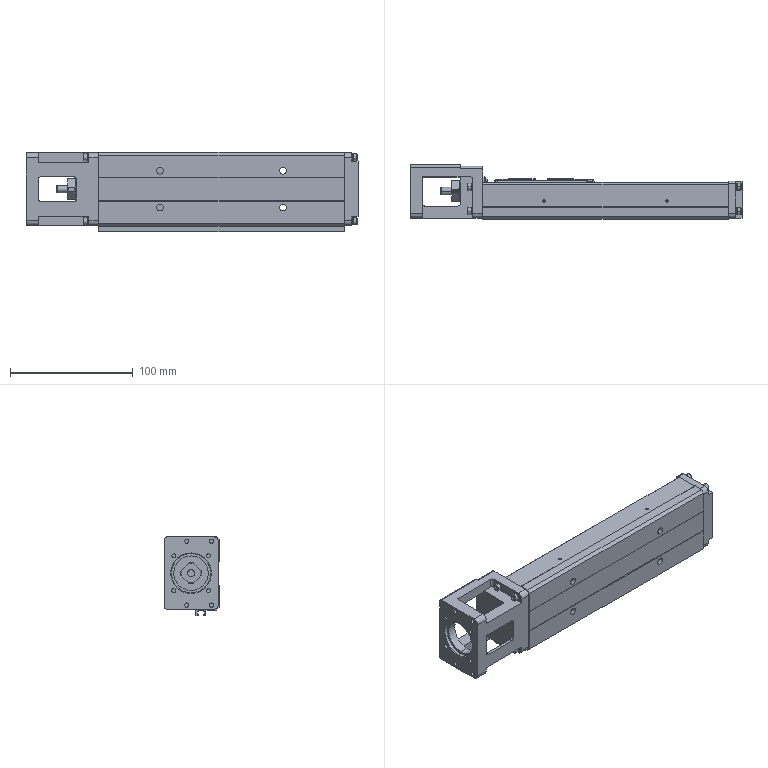Part | STEP file | Single-axis module KM3305A+200N0-013LCB | 3 solids | 2189 faces | box 270 x 44.5 x 64.6 mm | volume 342909 mm3 | plane 1782 | cylinder 279 | cone 88 | torus 22 | other 18 | commonest cylinder face diameters 6 x32 5.5 x28 8 x20 1 x18 4 x18 4.28 x16